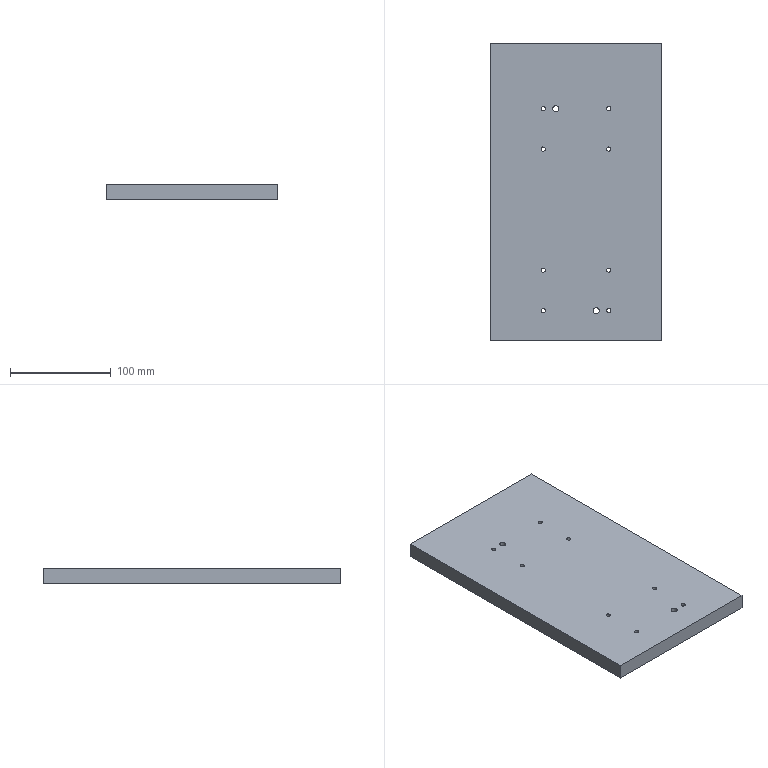Part | STEP file | SN10_012_002_PLACA | 1 solid | 16 faces | box 170 x 295 x 15 mm | volume 749791 mm3 | cylinder 10 | plane 6 | commonest cylinder face diameters 4.134 x8 6 x2
STEP:
#1=CARTESIAN_POINT('',(0.,0.,0.));
#2=DIRECTION('',(0.,0.,1.));
#3=DIRECTION('',(1.,0.,0.));
#4=AXIS2_PLACEMENT_3D('',#1,#2,#3);
#5=CARTESIAN_POINT('',(156.943,249.009,60.));
#6=VERTEX_POINT('',#5);
#7=CARTESIAN_POINT('',(155.129,250.,60.));
#8=DIRECTION('',(0.,0.,1.));
#9=DIRECTION('',(1.,0.,0.));
#10=AXIS2_PLACEMENT_3D('',#7,#8,#9);
#11=CIRCLE('',#10,2.067);
#12=CARTESIAN_POINT('',(155.129,250.,59.9));
#13=DIRECTION('',(0.,0.,-1.));
#14=DIRECTION('',(0.8776,-0.4794,0.));
#15=AXIS2_PLACEMENT_3D('',#12,#13,#14);
#16=CYLINDRICAL_SURFACE('',#15,2.067);
#17=CARTESIAN_POINT('',(12.066,-0.1));
#18=DIRECTION('',(-1.,0.));
#19=VECTOR('',#18,1.);
#20=LINE('',#17,#19);
#21=(GEOMETRIC_REPRESENTATION_CONTEXT(2)PARAMETRIC_REPRESENTATION_CONTEXT()REPRESENTATION_CONTEXT('',''));
#22=DEFINITIONAL_REPRESENTATION('',(#20),#21);
#23=PCURVE('',#16,#22);
#24=CARTESIAN_POINT('',(0.,0.,60.));
#25=DIRECTION('',(0.,0.,1.));
#26=DIRECTION('',(1.,0.,0.));
#27=AXIS2_PLACEMENT_3D('',#24,#25,#26);
#28=PLANE('',#27);
#29=CARTESIAN_POINT('',(155.129,250.));
#30=DIRECTION('',(1.,0.));
#31=AXIS2_PLACEMENT_2D('',#29,#30);
#32=CIRCLE('',#31,2.067);
#33=(GEOMETRIC_REPRESENTATION_CONTEXT(2)PARAMETRIC_REPRESENTATION_CONTEXT()REPRESENTATION_CONTEXT('',''));
#34=DEFINITIONAL_REPRESENTATION('',(#32),#33);
#35=PCURVE('',#28,#34);
#36=SURFACE_CURVE('',#11,(#23,#35),.PCURVE_S1.);
#37=EDGE_CURVE('',#6,#6,#36,.T.);
#38=ORIENTED_EDGE('',*,*,#37,.F.);
#39=CARTESIAN_POINT('',(156.943,249.009,45.));
#40=VERTEX_POINT('',#39);
#41=CARTESIAN_POINT('',(156.943,249.009,60.));
#42=CARTESIAN_POINT('',(156.943,249.009,45.));
#43=B_SPLINE_CURVE_WITH_KNOTS('',1,(#41,#42),.UNSPECIFIED.,.F.,.F.,(2,2),(-0.1,14.9),.PIECEWISE_BEZIER_KNOTS.);
#44=CARTESIAN_POINT('',(6.283,0.));
#45=DIRECTION('',(0.,1.));
#46=VECTOR('',#45,1.);
#47=LINE('',#44,#46);
#48=(GEOMETRIC_REPRESENTATION_CONTEXT(2)PARAMETRIC_REPRESENTATION_CONTEXT()REPRESENTATION_CONTEXT('',''));
#49=DEFINITIONAL_REPRESENTATION('',(#47),#48);
#50=PCURVE('',#16,#49);
#51=CARTESIAN_POINT('',(0.,0.));
#52=DIRECTION('',(0.,1.));
#53=VECTOR('',#52,1.);
#54=LINE('',#51,#53);
#55=(GEOMETRIC_REPRESENTATION_CONTEXT(2)PARAMETRIC_REPRESENTATION_CONTEXT()REPRESENTATION_CONTEXT('',''));
#56=DEFINITIONAL_REPRESENTATION('',(#54),#55);
#57=PCURVE('',#16,#56);
#58=SEAM_CURVE('',#43,(#50,#57),.PCURVE_S1.);
#59=EDGE_CURVE('',#6,#40,#58,.T.);
#60=ORIENTED_EDGE('',*,*,#59,.T.);
#61=CARTESIAN_POINT('',(155.129,250.,45.));
#62=DIRECTION('',(0.,0.,-1.));
#63=DIRECTION('',(1.,0.,0.));
#64=AXIS2_PLACEMENT_3D('',#61,#62,#63);
#65=CIRCLE('',#64,2.067);
#66=CARTESIAN_POINT('',(-0.5,14.9));
#67=DIRECTION('',(1.,0.));
#68=VECTOR('',#67,1.);
#69=LINE('',#66,#68);
#70=(GEOMETRIC_REPRESENTATION_CONTEXT(2)PARAMETRIC_REPRESENTATION_CONTEXT()REPRESENTATION_CONTEXT('',''));
#71=DEFINITIONAL_REPRESENTATION('',(#69),#70);
#72=PCURVE('',#16,#71);
#73=CARTESIAN_POINT('',(0.,0.,45.));
#74=DIRECTION('',(0.,0.,1.));
#75=DIRECTION('',(1.,0.,0.));
#76=AXIS2_PLACEMENT_3D('',#73,#74,#75);
#77=PLANE('',#76);
#78=CARTESIAN_POINT('',(157.196,250.));
#79=CARTESIAN_POINT('',(157.196,246.42));
#80=CARTESIAN_POINT('',(154.095,248.21));
#81=CARTESIAN_POINT('',(150.995,250.));
#82=CARTESIAN_POINT('',(154.095,251.79));
#83=CARTESIAN_POINT('',(157.196,253.58));
#84=CARTESIAN_POINT('',(157.196,250.));
#85=(BOUNDED_CURVE()B_SPLINE_CURVE(2,(#78,#79,#80,#81,#82,#83,#84),.UNSPECIFIED.,.T.,.F.)B_SPLINE_CURVE_WITH_KNOTS((1,2,2,2,2,1),(-2.094,0.,2.094,4.189,6.283,8.378),.UNSPECIFIED.)CURVE()GEOMETRIC_REPRESENTATION_ITEM()RATIONAL_B_SPLINE_CURVE((1.,0.5,1.,0.5,1.,0.5,1.))REPRESENTATION_ITEM(''));
#86=(GEOMETRIC_REPRESENTATION_CONTEXT(2)PARAMETRIC_REPRESENTATION_CONTEXT()REPRESENTATION_CONTEXT('',''));
#87=DEFINITIONAL_REPRESENTATION('',(#85),#86);
#88=PCURVE('',#77,#87);
#89=SURFACE_CURVE('',#65,(#72,#88),.PCURVE_S1.);
#90=EDGE_CURVE('',#40,#40,#89,.T.);
#91=ORIENTED_EDGE('',*,*,#90,.F.);
#92=ORIENTED_EDGE('',*,*,#59,.F.);
#93=EDGE_LOOP('',(#38,#60,#91,#92));
#94=FACE_BOUND('',#93,.F.);
#95=ADVANCED_FACE('',(#94),#16,.F.);
#96=CARTESIAN_POINT('',(102.629,475.,60.));
#97=VERTEX_POINT('',#96);
#98=CARTESIAN_POINT('',(102.629,180.,60.));
#99=VERTEX_POINT('',#98);
#100=CARTESIAN_POINT('',(102.629,475.,60.));
#101=DIRECTION('',(0.,-1.,0.));
#102=VECTOR('',#101,1.);
#103=LINE('',#100,#102);
#104=CARTESIAN_POINT('',(102.629,475.));
#105=DIRECTION('',(0.,-1.));
#106=VECTOR('',#105,1.);
#107=LINE('',#104,#106);
#108=(GEOMETRIC_REPRESENTATION_CONTEXT(2)PARAMETRIC_REPRESENTATION_CONTEXT()REPRESENTATION_CONTEXT('',''));
#109=DEFINITIONAL_REPRESENTATION('',(#107),#108);
#110=PCURVE('',#28,#109);
#111=CARTESIAN_POINT('',(102.629,475.,45.));
#112=DIRECTION('',(-1.,0.,0.));
#113=DIRECTION('',(0.,0.,1.));
#114=AXIS2_PLACEMENT_3D('',#111,#112,#113);
#115=PLANE('',#114);
#116=CARTESIAN_POINT('',(15.,0.));
#117=DIRECTION('',(0.,-1.));
#118=VECTOR('',#117,1.);
#119=LINE('',#116,#118);
#120=(GEOMETRIC_REPRESENTATION_CONTEXT(2)PARAMETRIC_REPRESENTATION_CONTEXT()REPRESENTATION_CONTEXT('',''));
#121=DEFINITIONAL_REPRESENTATION('',(#119),#120);
#122=PCURVE('',#115,#121);
#123=SURFACE_CURVE('',#103,(#110,#122),.PCURVE_S1.);
#124=EDGE_CURVE('',#97,#99,#123,.T.);
#125=ORIENTED_EDGE('',*,*,#124,.T.);
#126=CARTESIAN_POINT('',(272.629,180.,60.));
#127=VERTEX_POINT('',#126);
#128=CARTESIAN_POINT('',(272.629,180.,60.));
#129=DIRECTION('',(-1.,0.,0.));
#130=VECTOR('',#129,1.);
#131=LINE('',#128,#130);
#132=CARTESIAN_POINT('',(272.629,180.));
#133=DIRECTION('',(-1.,0.));
#134=VECTOR('',#133,1.);
#135=LINE('',#132,#134);
#136=(GEOMETRIC_REPRESENTATION_CONTEXT(2)PARAMETRIC_REPRESENTATION_CONTEXT()REPRESENTATION_CONTEXT('',''));
#137=DEFINITIONAL_REPRESENTATION('',(#135),#136);
#138=PCURVE('',#28,#137);
#139=CARTESIAN_POINT('',(272.629,180.,45.));
#140=DIRECTION('',(0.,1.,0.));
#141=DIRECTION('',(0.,0.,1.));
#142=AXIS2_PLACEMENT_3D('',#139,#140,#141);
#143=PLANE('',#142);
#144=CARTESIAN_POINT('',(15.,0.));
#145=DIRECTION('',(0.,-1.));
#146=VECTOR('',#145,1.);
#147=LINE('',#144,#146);
#148=(GEOMETRIC_REPRESENTATION_CONTEXT(2)PARAMETRIC_REPRESENTATION_CONTEXT()REPRESENTATION_CONTEXT('',''));
#149=DEFINITIONAL_REPRESENTATION('',(#147),#148);
#150=PCURVE('',#143,#149);
#151=SURFACE_CURVE('',#131,(#138,#150),.PCURVE_S1.);
#152=EDGE_CURVE('',#127,#99,#151,.T.);
#153=ORIENTED_EDGE('',*,*,#152,.F.);
#154=CARTESIAN_POINT('',(272.629,475.,60.));
#155=VERTEX_POINT('',#154);
#156=CARTESIAN_POINT('',(272.629,180.,60.));
#157=DIRECTION('',(0.,1.,0.));
#158=VECTOR('',#157,1.);
#159=LINE('',#156,#158);
#160=CARTESIAN_POINT('',(272.629,180.));
#161=DIRECTION('',(0.,1.));
#162=VECTOR('',#161,1.);
#163=LINE('',#160,#162);
#164=(GEOMETRIC_REPRESENTATION_CONTEXT(2)PARAMETRIC_REPRESENTATION_CONTEXT()REPRESENTATION_CONTEXT('',''));
#165=DEFINITIONAL_REPRESENTATION('',(#163),#164);
#166=PCURVE('',#28,#165);
#167=CARTESIAN_POINT('',(272.629,180.,45.));
#168=DIRECTION('',(1.,0.,0.));
#169=DIRECTION('',(0.,0.,-1.));
#170=AXIS2_PLACEMENT_3D('',#167,#168,#169);
#171=PLANE('',#170);
#172=CARTESIAN_POINT('',(-15.,0.));
#173=DIRECTION('',(0.,1.));
#174=VECTOR('',#173,1.);
#175=LINE('',#172,#174);
#176=(GEOMETRIC_REPRESENTATION_CONTEXT(2)PARAMETRIC_REPRESENTATION_CONTEXT()REPRESENTATION_CONTEXT('',''));
#177=DEFINITIONAL_REPRESENTATION('',(#175),#176);
#178=PCURVE('',#171,#177);
#179=SURFACE_CURVE('',#159,(#166,#178),.PCURVE_S1.);
#180=EDGE_CURVE('',#127,#155,#179,.T.);
#181=ORIENTED_EDGE('',*,*,#180,.T.);
#182=CARTESIAN_POINT('',(102.629,475.,60.));
#183=DIRECTION('',(1.,0.,0.));
#184=VECTOR('',#183,1.);
#185=LINE('',#182,#184);
#186=CARTESIAN_POINT('',(102.629,475.));
#187=DIRECTION('',(1.,0.));
#188=VECTOR('',#187,1.);
#189=LINE('',#186,#188);
#190=(GEOMETRIC_REPRESENTATION_CONTEXT(2)PARAMETRIC_REPRESENTATION_CONTEXT()REPRESENTATION_CONTEXT('',''));
#191=DEFINITIONAL_REPRESENTATION('',(#189),#190);
#192=PCURVE('',#28,#191);
#193=CARTESIAN_POINT('',(102.629,475.,45.));
#194=DIRECTION('',(0.,-1.,0.));
#195=DIRECTION('',(0.,0.,-1.));
#196=AXIS2_PLACEMENT_3D('',#193,#194,#195);
#197=PLANE('',#196);
#198=CARTESIAN_POINT('',(-15.,0.));
#199=DIRECTION('',(0.,1.));
#200=VECTOR('',#199,1.);
#201=LINE('',#198,#200);
#202=(GEOMETRIC_REPRESENTATION_CONTEXT(2)PARAMETRIC_REPRESENTATION_CONTEXT()REPRESENTATION_CONTEXT('',''));
#203=DEFINITIONAL_REPRESENTATION('',(#201),#202);
#204=PCURVE('',#197,#203);
#205=SURFACE_CURVE('',#185,(#192,#204),.PCURVE_S1.);
#206=EDGE_CURVE('',#97,#155,#205,.T.);
#207=ORIENTED_EDGE('',*,*,#206,.F.);
#208=EDGE_LOOP('',(#125,#153,#181,#207));
#209=FACE_BOUND('',#208,.T.);
#210=ORIENTED_EDGE('',*,*,#37,.F.);
#211=EDGE_LOOP('',(#210));
#212=FACE_BOUND('',#211,.T.);
#213=CARTESIAN_POINT('',(156.943,209.009,60.));
#214=VERTEX_POINT('',#213);
#215=CARTESIAN_POINT('',(155.129,210.,60.));
#216=DIRECTION('',(0.,0.,1.));
#217=DIRECTION('',(1.,0.,0.));
#218=AXIS2_PLACEMENT_3D('',#215,#216,#217);
#219=CIRCLE('',#218,2.067);
#220=CARTESIAN_POINT('',(155.129,210.));
#221=DIRECTION('',(1.,0.));
#222=AXIS2_PLACEMENT_2D('',#220,#221);
#223=CIRCLE('',#222,2.067);
#224=(GEOMETRIC_REPRESENTATION_CONTEXT(2)PARAMETRIC_REPRESENTATION_CONTEXT()REPRESENTATION_CONTEXT('',''));
#225=DEFINITIONAL_REPRESENTATION('',(#223),#224);
#226=PCURVE('',#28,#225);
#227=CARTESIAN_POINT('',(155.129,210.,59.9));
#228=DIRECTION('',(0.,0.,-1.));
#229=DIRECTION('',(0.8776,-0.4794,0.));
#230=AXIS2_PLACEMENT_3D('',#227,#228,#229);
#231=CYLINDRICAL_SURFACE('',#230,2.067);
#232=CARTESIAN_POINT('',(12.066,-0.1));
#233=DIRECTION('',(-1.,0.));
#234=VECTOR('',#233,1.);
#235=LINE('',#232,#234);
#236=(GEOMETRIC_REPRESENTATION_CONTEXT(2)PARAMETRIC_REPRESENTATION_CONTEXT()REPRESENTATION_CONTEXT('',''));
#237=DEFINITIONAL_REPRESENTATION('',(#235),#236);
#238=PCURVE('',#231,#237);
#239=SURFACE_CURVE('',#219,(#226,#238),.PCURVE_S1.);
#240=EDGE_CURVE('',#214,#214,#239,.T.);
#241=ORIENTED_EDGE('',*,*,#240,.F.);
#242=EDGE_LOOP('',(#241));
#243=FACE_BOUND('',#242,.T.);
#244=CARTESIAN_POINT('',(221.943,209.009,60.));
#245=VERTEX_POINT('',#244);
#246=CARTESIAN_POINT('',(220.129,210.,60.));
#247=DIRECTION('',(0.,0.,1.));
#248=DIRECTION('',(1.,0.,0.));
#249=AXIS2_PLACEMENT_3D('',#246,#247,#248);
#250=CIRCLE('',#249,2.067);
#251=CARTESIAN_POINT('',(220.129,210.));
#252=DIRECTION('',(1.,0.));
#253=AXIS2_PLACEMENT_2D('',#251,#252);
#254=CIRCLE('',#253,2.067);
#255=(GEOMETRIC_REPRESENTATION_CONTEXT(2)PARAMETRIC_REPRESENTATION_CONTEXT()REPRESENTATION_CONTEXT('',''));
#256=DEFINITIONAL_REPRESENTATION('',(#254),#255);
#257=PCURVE('',#28,#256);
#258=CARTESIAN_POINT('',(220.129,210.,59.9));
#259=DIRECTION('',(0.,0.,-1.));
#260=DIRECTION('',(0.8776,-0.4794,0.));
#261=AXIS2_PLACEMENT_3D('',#258,#259,#260);
#262=CYLINDRICAL_SURFACE('',#261,2.067);
#263=CARTESIAN_POINT('',(12.066,-0.1));
#264=DIRECTION('',(-1.,0.));
#265=VECTOR('',#264,1.);
#266=LINE('',#263,#265);
#267=(GEOMETRIC_REPRESENTATION_CONTEXT(2)PARAMETRIC_REPRESENTATION_CONTEXT()REPRESENTATION_CONTEXT('',''));
#268=DEFINITIONAL_REPRESENTATION('',(#266),#267);
#269=PCURVE('',#262,#268);
#270=SURFACE_CURVE('',#250,(#257,#269),.PCURVE_S1.);
#271=EDGE_CURVE('',#245,#245,#270,.T.);
#272=ORIENTED_EDGE('',*,*,#271,.F.);
#273=EDGE_LOOP('',(#272));
#274=FACE_BOUND('',#273,.T.);
#275=CARTESIAN_POINT('',(221.943,249.009,60.));
#276=VERTEX_POINT('',#275);
#277=CARTESIAN_POINT('',(220.129,250.,60.));
#278=DIRECTION('',(0.,0.,1.));
#279=DIRECTION('',(1.,0.,0.));
#280=AXIS2_PLACEMENT_3D('',#277,#278,#279);
#281=CIRCLE('',#280,2.067);
#282=CARTESIAN_POINT('',(220.129,250.));
#283=DIRECTION('',(1.,0.));
#284=AXIS2_PLACEMENT_2D('',#282,#283);
#285=CIRCLE('',#284,2.067);
#286=(GEOMETRIC_REPRESENTATION_CONTEXT(2)PARAMETRIC_REPRESENTATION_CONTEXT()REPRESENTATION_CONTEXT('',''));
#287=DEFINITIONAL_REPRESENTATION('',(#285),#286);
#288=PCURVE('',#28,#287);
#289=CARTESIAN_POINT('',(220.129,250.,59.9));
#290=DIRECTION('',(0.,0.,-1.));
#291=DIRECTION('',(0.8776,-0.4794,0.));
#292=AXIS2_PLACEMENT_3D('',#289,#290,#291);
#293=CYLINDRICAL_SURFACE('',#292,2.067);
#294=CARTESIAN_POINT('',(12.066,-0.1));
#295=DIRECTION('',(-1.,0.));
#296=VECTOR('',#295,1.);
#297=LINE('',#294,#296);
#298=(GEOMETRIC_REPRESENTATION_CONTEXT(2)PARAMETRIC_REPRESENTATION_CONTEXT()REPRESENTATION_CONTEXT('',''));
#299=DEFINITIONAL_REPRESENTATION('',(#297),#298);
#300=PCURVE('',#293,#299);
#301=SURFACE_CURVE('',#281,(#288,#300),.PCURVE_S1.);
#302=EDGE_CURVE('',#276,#276,#301,.T.);
#303=ORIENTED_EDGE('',*,*,#302,.F.);
#304=EDGE_LOOP('',(#303));
#305=FACE_BOUND('',#304,.T.);
#306=CARTESIAN_POINT('',(221.943,369.009,60.));
#307=VERTEX_POINT('',#306);
#308=CARTESIAN_POINT('',(220.129,370.,60.));
#309=DIRECTION('',(0.,0.,1.));
#310=DIRECTION('',(1.,0.,0.));
#311=AXIS2_PLACEMENT_3D('',#308,#309,#310);
#312=CIRCLE('',#311,2.067);
#313=CARTESIAN_POINT('',(220.129,370.));
#314=DIRECTION('',(1.,0.));
#315=AXIS2_PLACEMENT_2D('',#313,#314);
#316=CIRCLE('',#315,2.067);
#317=(GEOMETRIC_REPRESENTATION_CONTEXT(2)PARAMETRIC_REPRESENTATION_CONTEXT()REPRESENTATION_CONTEXT('',''));
#318=DEFINITIONAL_REPRESENTATION('',(#316),#317);
#319=PCURVE('',#28,#318);
#320=CARTESIAN_POINT('',(220.129,370.,59.9));
#321=DIRECTION('',(0.,0.,-1.));
#322=DIRECTION('',(0.8776,-0.4794,0.));
#323=AXIS2_PLACEMENT_3D('',#320,#321,#322);
#324=CYLINDRICAL_SURFACE('',#323,2.067);
#325=CARTESIAN_POINT('',(12.066,-0.1));
#326=DIRECTION('',(-1.,0.));
#327=VECTOR('',#326,1.);
#328=LINE('',#325,#327);
#329=(GEOMETRIC_REPRESENTATION_CONTEXT(2)PARAMETRIC_REPRESENTATION_CONTEXT()REPRESENTATION_CONTEXT('',''));
#330=DEFINITIONAL_REPRESENTATION('',(#328),#329);
#331=PCURVE('',#324,#330);
#332=SURFACE_CURVE('',#312,(#319,#331),.PCURVE_S1.);
#333=EDGE_CURVE('',#307,#307,#332,.T.);
#334=ORIENTED_EDGE('',*,*,#333,.F.);
#335=EDGE_LOOP('',(#334));
#336=FACE_BOUND('',#335,.T.);
#337=CARTESIAN_POINT('',(156.943,369.009,60.));
#338=VERTEX_POINT('',#337);
#339=CARTESIAN_POINT('',(155.129,370.,60.));
#340=DIRECTION('',(0.,0.,1.));
#341=DIRECTION('',(1.,0.,0.));
#342=AXIS2_PLACEMENT_3D('',#339,#340,#341);
#343=CIRCLE('',#342,2.067);
#344=CARTESIAN_POINT('',(155.129,370.));
#345=DIRECTION('',(1.,0.));
#346=AXIS2_PLACEMENT_2D('',#344,#345);
#347=CIRCLE('',#346,2.067);
#348=(GEOMETRIC_REPRESENTATION_CONTEXT(2)PARAMETRIC_REPRESENTATION_CONTEXT()REPRESENTATION_CONTEXT('',''));
#349=DEFINITIONAL_REPRESENTATION('',(#347),#348);
#350=PCURVE('',#28,#349);
#351=CARTESIAN_POINT('',(155.129,370.,59.9));
#352=DIRECTION('',(0.,0.,-1.));
#353=DIRECTION('',(0.8776,-0.4794,0.));
#354=AXIS2_PLACEMENT_3D('',#351,#352,#353);
#355=CYLINDRICAL_SURFACE('',#354,2.067);
#356=CARTESIAN_POINT('',(12.066,-0.1));
#357=DIRECTION('',(-1.,0.));
#358=VECTOR('',#357,1.);
#359=LINE('',#356,#358);
#360=(GEOMETRIC_REPRESENTATION_CONTEXT(2)PARAMETRIC_REPRESENTATION_CONTEXT()REPRESENTATION_CONTEXT('',''));
#361=DEFINITIONAL_REPRESENTATION('',(#359),#360);
#362=PCURVE('',#355,#361);
#363=SURFACE_CURVE('',#343,(#350,#362),.PCURVE_S1.);
#364=EDGE_CURVE('',#338,#338,#363,.T.);
#365=ORIENTED_EDGE('',*,*,#364,.F.);
#366=EDGE_LOOP('',(#365));
#367=FACE_BOUND('',#366,.T.);
#368=CARTESIAN_POINT('',(156.943,409.009,60.));
#369=VERTEX_POINT('',#368);
#370=CARTESIAN_POINT('',(155.129,410.,60.));
#371=DIRECTION('',(0.,0.,1.));
#372=DIRECTION('',(1.,0.,0.));
#373=AXIS2_PLACEMENT_3D('',#370,#371,#372);
#374=CIRCLE('',#373,2.067);
#375=CARTESIAN_POINT('',(155.129,410.));
#376=DIRECTION('',(1.,0.));
#377=AXIS2_PLACEMENT_2D('',#375,#376);
#378=CIRCLE('',#377,2.067);
#379=(GEOMETRIC_REPRESENTATION_CONTEXT(2)PARAMETRIC_REPRESENTATION_CONTEXT()REPRESENTATION_CONTEXT('',''));
#380=DEFINITIONAL_REPRESENTATION('',(#378),#379);
#381=PCURVE('',#28,#380);
#382=CARTESIAN_POINT('',(155.129,410.,59.9));
#383=DIRECTION('',(0.,0.,-1.));
#384=DIRECTION('',(0.8776,-0.4794,0.));
#385=AXIS2_PLACEMENT_3D('',#382,#383,#384);
#386=CYLINDRICAL_SURFACE('',#385,2.067);
#387=CARTESIAN_POINT('',(12.066,-0.1));
#388=DIRECTION('',(-1.,0.));
#389=VECTOR('',#388,1.);
#390=LINE('',#387,#389);
#391=(GEOMETRIC_REPRESENTATION_CONTEXT(2)PARAMETRIC_REPRESENTATION_CONTEXT()REPRESENTATION_CONTEXT('',''));
#392=DEFINITIONAL_REPRESENTATION('',(#390),#391);
#393=PCURVE('',#386,#392);
#394=SURFACE_CURVE('',#374,(#381,#393),.PCURVE_S1.);
#395=EDGE_CURVE('',#369,#369,#394,.T.);
#396=ORIENTED_EDGE('',*,*,#395,.F.);
#397=EDGE_LOOP('',(#396));
#398=FACE_BOUND('',#397,.T.);
#399=CARTESIAN_POINT('',(221.943,409.009,60.));
#400=VERTEX_POINT('',#399);
#401=CARTESIAN_POINT('',(220.129,410.,60.));
#402=DIRECTION('',(0.,0.,1.));
#403=DIRECTION('',(1.,0.,0.));
#404=AXIS2_PLACEMENT_3D('',#401,#402,#403);
#405=CIRCLE('',#404,2.067);
#406=CARTESIAN_POINT('',(220.129,410.));
#407=DIRECTION('',(1.,0.));
#408=AXIS2_PLACEMENT_2D('',#406,#407);
#409=CIRCLE('',#408,2.067);
#410=(GEOMETRIC_REPRESENTATION_CONTEXT(2)PARAMETRIC_REPRESENTATION_CONTEXT()REPRESENTATION_CONTEXT('',''));
#411=DEFINITIONAL_REPRESENTATION('',(#409),#410);
#412=PCURVE('',#28,#411);
#413=CARTESIAN_POINT('',(220.129,410.,59.9));
#414=DIRECTION('',(0.,0.,-1.));
#415=DIRECTION('',(0.8776,-0.4794,0.));
#416=AXIS2_PLACEMENT_3D('',#413,#414,#415);
#417=CYLINDRICAL_SURFACE('',#416,2.067);
#418=CARTESIAN_POINT('',(12.066,-0.1));
#419=DIRECTION('',(-1.,0.));
#420=VECTOR('',#419,1.);
#421=LINE('',#418,#420);
#422=(GEOMETRIC_REPRESENTATION_CONTEXT(2)PARAMETRIC_REPRESENTATION_CONTEXT()REPRESENTATION_CONTEXT('',''));
#423=DEFINITIONAL_REPRESENTATION('',(#421),#422);
#424=PCURVE('',#417,#423);
#425=SURFACE_CURVE('',#405,(#412,#424),.PCURVE_S1.);
#426=EDGE_CURVE('',#400,#400,#425,.T.);
#427=ORIENTED_EDGE('',*,*,#426,.F.);
#428=EDGE_LOOP('',(#427));
#429=FACE_BOUND('',#428,.T.);
#430=CARTESIAN_POINT('',(210.262,208.562,60.));
#431=VERTEX_POINT('',#430);
#432=CARTESIAN_POINT('',(207.629,210.,60.));
#433=DIRECTION('',(0.,0.,1.));
#434=DIRECTION('',(1.,0.,0.));
#435=AXIS2_PLACEMENT_3D('',#432,#433,#434);
#436=CIRCLE('',#435,3.);
#437=CARTESIAN_POINT('',(207.629,210.));
#438=DIRECTION('',(1.,0.));
#439=AXIS2_PLACEMENT_2D('',#437,#438);
#440=CIRCLE('',#439,3.);
#441=(GEOMETRIC_REPRESENTATION_CONTEXT(2)PARAMETRIC_REPRESENTATION_CONTEXT()REPRESENTATION_CONTEXT('',''));
#442=DEFINITIONAL_REPRESENTATION('',(#440),#441);
#443=PCURVE('',#28,#442);
#444=CARTESIAN_POINT('',(207.629,210.,59.9));
#445=DIRECTION('',(0.,0.,-1.));
#446=DIRECTION('',(0.8776,-0.4794,0.));
#447=AXIS2_PLACEMENT_3D('',#444,#445,#446);
#448=CYLINDRICAL_SURFACE('',#447,3.);
#449=CARTESIAN_POINT('',(12.066,-0.1));
#450=DIRECTION('',(-1.,0.));
#451=VECTOR('',#450,1.);
#452=LINE('',#449,#451);
#453=(GEOMETRIC_REPRESENTATION_CONTEXT(2)PARAMETRIC_REPRESENTATION_CONTEXT()REPRESENTATION_CONTEXT('',''));
#454=DEFINITIONAL_REPRESENTATION('',(#452),#453);
#455=PCURVE('',#448,#454);
#456=SURFACE_CURVE('',#436,(#443,#455),.PCURVE_S1.);
#457=EDGE_CURVE('',#431,#431,#456,.T.);
#458=ORIENTED_EDGE('',*,*,#457,.F.);
#459=EDGE_LOOP('',(#458));
#460=FACE_BOUND('',#459,.T.);
#461=CARTESIAN_POINT('',(170.262,408.562,60.));
#462=VERTEX_POINT('',#461);
#463=CARTESIAN_POINT('',(167.629,410.,60.));
#464=DIRECTION('',(0.,0.,1.));
#465=DIRECTION('',(1.,0.,0.));
#466=AXIS2_PLACEMENT_3D('',#463,#464,#465);
#467=CIRCLE('',#466,3.);
#468=CARTESIAN_POINT('',(167.629,410.));
#469=DIRECTION('',(1.,0.));
#470=AXIS2_PLACEMENT_2D('',#468,#469);
#471=CIRCLE('',#470,3.);
#472=(GEOMETRIC_REPRESENTATION_CONTEXT(2)PARAMETRIC_REPRESENTATION_CONTEXT()REPRESENTATION_CONTEXT('',''));
#473=DEFINITIONAL_REPRESENTATION('',(#471),#472);
#474=PCURVE('',#28,#473);
#475=CARTESIAN_POINT('',(167.629,410.,59.9));
#476=DIRECTION('',(0.,0.,-1.));
#477=DIRECTION('',(0.8776,-0.4794,0.));
#478=AXIS2_PLACEMENT_3D('',#475,#476,#477);
#479=CYLINDRICAL_SURFACE('',#478,3.);
#480=CARTESIAN_POINT('',(12.066,-0.1));
#481=DIRECTION('',(-1.,0.));
#482=VECTOR('',#481,1.);
#483=LINE('',#480,#482);
#484=(GEOMETRIC_REPRESENTATION_CONTEXT(2)PARAMETRIC_REPRESENTATION_CONTEXT()REPRESENTATION_CONTEXT('',''));
#485=DEFINITIONAL_REPRESENTATION('',(#483),#484);
#486=PCURVE('',#479,#485);
#487=SURFACE_CURVE('',#467,(#474,#486),.PCURVE_S1.);
#488=EDGE_CURVE('',#462,#462,#487,.T.);
#489=ORIENTED_EDGE('',*,*,#488,.F.);
#490=EDGE_LOOP('',(#489));
#491=FACE_BOUND('',#490,.T.);
#492=ADVANCED_FACE('',(#209,#212,#243,#274,#305,#336,#367,#398,#429,#460,#491),#28,.T.);
#493=CARTESIAN_POINT('',(102.629,475.,45.));
#494=VERTEX_POINT('',#493);
#495=CARTESIAN_POINT('',(102.629,475.,45.));
#496=DIRECTION('',(0.,0.,1.));
#497=VECTOR('',#496,1.);
#498=LINE('',#495,#497);
#499=CARTESIAN_POINT('',(0.,0.));
#500=DIRECTION('',(1.,0.));
#501=VECTOR('',#500,1.);
#502=LINE('',#499,#501);
#503=(GEOMETRIC_REPRESENTATION_CONTEXT(2)PARAMETRIC_REPRESENTATION_CONTEXT()REPRESENTATION_CONTEXT('',''));
#504=DEFINITIONAL_REPRESENTATION('',(#502),#503);
#505=PCURVE('',#115,#504);
#506=CARTESIAN_POINT('',(0.,0.));
#507=DIRECTION('',(-1.,0.));
#508=VECTOR('',#507,1.);
#509=LINE('',#506,#508);
#510=(GEOMETRIC_REPRESENTATION_CONTEXT(2)PARAMETRIC_REPRESENTATION_CONTEXT()REPRESENTATION_CONTEXT('',''));
#511=DEFINITIONAL_REPRESENTATION('',(#509),#510);
#512=PCURVE('',#197,#511);
#513=SURFACE_CURVE('',#498,(#505,#512),.PCURVE_S1.);
#514=EDGE_CURVE('',#494,#97,#513,.T.);
#515=ORIENTED_EDGE('',*,*,#514,.F.);
#516=CARTESIAN_POINT('',(102.629,180.,45.));
#517=VERTEX_POINT('',#516);
#518=CARTESIAN_POINT('',(102.629,475.,45.));
#519=DIRECTION('',(0.,-1.,0.));
#520=VECTOR('',#519,1.);
#521=LINE('',#518,#520);
#522=CARTESIAN_POINT('',(0.,0.));
#523=DIRECTION('',(0.,-1.));
#524=VECTOR('',#523,1.);
#525=LINE('',#522,#524);
#526=(GEOMETRIC_REPRESENTATION_CONTEXT(2)PARAMETRIC_REPRESENTATION_CONTEXT()REPRESENTATION_CONTEXT('',''));
#527=DEFINITIONAL_REPRESENTATION('',(#525),#526);
#528=PCURVE('',#115,#527);
#529=CARTESIAN_POINT('',(102.629,475.));
#530=DIRECTION('',(0.,-1.));
#531=VECTOR('',#530,1.);
#532=LINE('',#529,#531);
#533=(GEOMETRIC_REPRESENTATION_CONTEXT(2)PARAMETRIC_REPRESENTATION_CONTEXT()REPRESENTATION_CONTEXT('',''));
#534=DEFINITIONAL_REPRESENTATION('',(#532),#533);
#535=PCURVE('',#77,#534);
#536=SURFACE_CURVE('',#521,(#528,#535),.PCURVE_S1.);
#537=EDGE_CURVE('',#494,#517,#536,.T.);
#538=ORIENTED_EDGE('',*,*,#537,.T.);
#539=CARTESIAN_POINT('',(102.629,180.,45.));
#540=DIRECTION('',(0.,0.,1.));
#541=VECTOR('',#540,1.);
#542=LINE('',#539,#541);
#543=CARTESIAN_POINT('',(0.,-295.));
#544=DIRECTION('',(1.,0.));
#545=VECTOR('',#544,1.);
#546=LINE('',#543,#545);
#547=(GEOMETRIC_REPRESENTATION_CONTEXT(2)PARAMETRIC_REPRESENTATION_CONTEXT()REPRESENTATION_CONTEXT('',''));
#548=DEFINITIONAL_REPRESENTATION('',(#546),#547);
#549=PCURVE('',#115,#548);
#550=CARTESIAN_POINT('',(0.,-170.));
#551=DIRECTION('',(1.,0.));
#552=VECTOR('',#551,1.);
#553=LINE('',#550,#552);
#554=(GEOMETRIC_REPRESENTATION_CONTEXT(2)PARAMETRIC_REPRESENTATION_CONTEXT()REPRESENTATION_CONTEXT('',''));
#555=DEFINITIONAL_REPRESENTATION('',(#553),#554);
#556=PCURVE('',#143,#555);
#557=SURFACE_CURVE('',#542,(#549,#556),.PCURVE_S1.);
#558=EDGE_CURVE('',#517,#99,#557,.T.);
#559=ORIENTED_EDGE('',*,*,#558,.T.);
#560=ORIENTED_EDGE('',*,*,#124,.F.);
#561=EDGE_LOOP('',(#515,#538,#559,#560));
#562=FACE_BOUND('',#561,.T.);
#563=ADVANCED_FACE('',(#562),#115,.T.);
#564=ORIENTED_EDGE('',*,*,#558,.F.);
#565=CARTESIAN_POINT('',(272.629,180.,45.));
#566=VERTEX_POINT('',#565);
#567=CARTESIAN_POINT('',(272.629,180.,45.));
#568=DIRECTION('',(-1.,0.,0.));
#569=VECTOR('',#568,1.);
#570=LINE('',#567,#569);
#571=CARTESIAN_POINT('',(0.,0.));
#572=DIRECTION('',(0.,-1.));
#573=VECTOR('',#572,1.);
#574=LINE('',#571,#573);
#575=(GEOMETRIC_REPRESENTATION_CONTEXT(2)PARAMETRIC_REPRESENTATION_CONTEXT()REPRESENTATION_CONTEXT('',''));
#576=DEFINITIONAL_REPRESENTATION('',(#574),#575);
#577=PCURVE('',#143,#576);
#578=CARTESIAN_POINT('',(272.629,180.));
#579=DIRECTION('',(-1.,0.));
#580=VECTOR('',#579,1.);
#581=LINE('',#578,#580);
#582=(GEOMETRIC_REPRESENTATION_CONTEXT(2)PARAMETRIC_REPRESENTATION_CONTEXT()REPRESENTATION_CONTEXT('',''));
#583=DEFINITIONAL_REPRESENTATION('',(#581),#582);
#584=PCURVE('',#77,#583);
#585=SURFACE_CURVE('',#570,(#577,#584),.PCURVE_S1.);
#586=EDGE_CURVE('',#566,#517,#585,.T.);
#587=ORIENTED_EDGE('',*,*,#586,.F.);
#588=CARTESIAN_POINT('',(272.629,180.,45.));
#589=DIRECTION('',(0.,0.,1.));
#590=VECTOR('',#589,1.);
#591=LINE('',#588,#590);
#592=CARTESIAN_POINT('',(0.,0.));
#593=DIRECTION('',(1.,0.));
#594=VECTOR('',#593,1.);
#595=LINE('',#592,#594);
#596=(GEOMETRIC_REPRESENTATION_CONTEXT(2)PARAMETRIC_REPRESENTATION_CONTEXT()REPRESENTATION_CONTEXT('',''));
#597=DEFINITIONAL_REPRESENTATION('',(#595),#596);
#598=PCURVE('',#143,#597);
#599=CARTESIAN_POINT('',(0.,0.));
#600=DIRECTION('',(-1.,0.));
#601=VECTOR('',#600,1.);
#602=LINE('',#599,#601);
#603=(GEOMETRIC_REPRESENTATION_CONTEXT(2)PARAMETRIC_REPRESENTATION_CONTEXT()REPRESENTATION_CONTEXT('',''));
#604=DEFINITIONAL_REPRESENTATION('',(#602),#603);
#605=PCURVE('',#171,#604);
#606=SURFACE_CURVE('',#591,(#598,#605),.PCURVE_S1.);
#607=EDGE_CURVE('',#566,#127,#606,.T.);
#608=ORIENTED_EDGE('',*,*,#607,.T.);
#609=ORIENTED_EDGE('',*,*,#152,.T.);
#610=EDGE_LOOP('',(#564,#587,#608,#609));
#611=FACE_BOUND('',#610,.T.);
#612=ADVANCED_FACE('',(#611),#143,.F.);
#613=ORIENTED_EDGE('',*,*,#607,.F.);
#614=CARTESIAN_POINT('',(272.629,475.,45.));
#615=VERTEX_POINT('',#614);
#616=CARTESIAN_POINT('',(272.629,180.,45.));
#617=DIRECTION('',(0.,1.,0.));
#618=VECTOR('',#617,1.);
#619=LINE('',#616,#618);
#620=CARTESIAN_POINT('',(0.,0.));
#621=DIRECTION('',(0.,1.));
#622=VECTOR('',#621,1.);
#623=LINE('',#620,#622);
#624=(GEOMETRIC_REPRESENTATION_CONTEXT(2)PARAMETRIC_REPRESENTATION_CONTEXT()REPRESENTATION_CONTEXT('',''));
#625=DEFINITIONAL_REPRESENTATION('',(#623),#624);
#626=PCURVE('',#171,#625);
#627=CARTESIAN_POINT('',(272.629,180.));
#628=DIRECTION('',(0.,1.));
#629=VECTOR('',#628,1.);
#630=LINE('',#627,#629);
#631=(GEOMETRIC_REPRESENTATION_CONTEXT(2)PARAMETRIC_REPRESENTATION_CONTEXT()REPRESENTATION_CONTEXT('',''));
#632=DEFINITIONAL_REPRESENTATION('',(#630),#631);
#633=PCURVE('',#77,#632);
#634=SURFACE_CURVE('',#619,(#626,#633),.PCURVE_S1.);
#635=EDGE_CURVE('',#566,#615,#634,.T.);
#636=ORIENTED_EDGE('',*,*,#635,.T.);
#637=CARTESIAN_POINT('',(272.629,475.,45.));
#638=DIRECTION('',(0.,0.,1.));
#639=VECTOR('',#638,1.);
#640=LINE('',#637,#639);
#641=CARTESIAN_POINT('',(0.,295.));
#642=DIRECTION('',(-1.,0.));
#643=VECTOR('',#642,1.);
#644=LINE('',#641,#643);
#645=(GEOMETRIC_REPRESENTATION_CONTEXT(2)PARAMETRIC_REPRESENTATION_CONTEXT()REPRESENTATION_CONTEXT('',''));
#646=DEFINITIONAL_REPRESENTATION('',(#644),#645);
#647=PCURVE('',#171,#646);
#648=CARTESIAN_POINT('',(0.,170.));
#649=DIRECTION('',(-1.,0.));
#650=VECTOR('',#649,1.);
#651=LINE('',#648,#650);
#652=(GEOMETRIC_REPRESENTATION_CONTEXT(2)PARAMETRIC_REPRESENTATION_CONTEXT()REPRESENTATION_CONTEXT('',''));
#653=DEFINITIONAL_REPRESENTATION('',(#651),#652);
#654=PCURVE('',#197,#653);
#655=SURFACE_CURVE('',#640,(#647,#654),.PCURVE_S1.);
#656=EDGE_CURVE('',#615,#155,#655,.T.);
#657=ORIENTED_EDGE('',*,*,#656,.T.);
#658=ORIENTED_EDGE('',*,*,#180,.F.);
#659=EDGE_LOOP('',(#613,#636,#657,#658));
#660=FACE_BOUND('',#659,.T.);
#661=ADVANCED_FACE('',(#660),#171,.T.);
#662=ORIENTED_EDGE('',*,*,#656,.F.);
#663=CARTESIAN_POINT('',(102.629,475.,45.));
#664=DIRECTION('',(1.,0.,0.));
#665=VECTOR('',#664,1.);
#666=LINE('',#663,#665);
#667=CARTESIAN_POINT('',(0.,0.));
#668=DIRECTION('',(0.,1.));
#669=VECTOR('',#668,1.);
#670=LINE('',#667,#669);
#671=(GEOMETRIC_REPRESENTATION_CONTEXT(2)PARAMETRIC_REPRESENTATION_CONTEXT()REPRESENTATION_CONTEXT('',''));
#672=DEFINITIONAL_REPRESENTATION('',(#670),#671);
#673=PCURVE('',#197,#672);
#674=CARTESIAN_POINT('',(102.629,475.));
#675=DIRECTION('',(1.,0.));
#676=VECTOR('',#675,1.);
#677=LINE('',#674,#676);
#678=(GEOMETRIC_REPRESENTATION_CONTEXT(2)PARAMETRIC_REPRESENTATION_CONTEXT()REPRESENTATION_CONTEXT('',''));
#679=DEFINITIONAL_REPRESENTATION('',(#677),#678);
#680=PCURVE('',#77,#679);
#681=SURFACE_CURVE('',#666,(#673,#680),.PCURVE_S1.);
#682=EDGE_CURVE('',#494,#615,#681,.T.);
#683=ORIENTED_EDGE('',*,*,#682,.F.);
#684=ORIENTED_EDGE('',*,*,#514,.T.);
#685=ORIENTED_EDGE('',*,*,#206,.T.);
#686=EDGE_LOOP('',(#662,#683,#684,#685));
#687=FACE_BOUND('',#686,.T.);
#688=ADVANCED_FACE('',(#687),#197,.F.);
#689=ORIENTED_EDGE('',*,*,#488,.F.);
#690=CARTESIAN_POINT('',(170.262,408.562,45.));
#691=VERTEX_POINT('',#690);
#692=CARTESIAN_POINT('',(170.262,408.562,60.));
#693=CARTESIAN_POINT('',(170.262,408.562,45.));
#694=B_SPLINE_CURVE_WITH_KNOTS('',1,(#692,#693),.UNSPECIFIED.,.F.,.F.,(2,2),(-0.1,14.9),.PIECEWISE_BEZIER_KNOTS.);
#695=CARTESIAN_POINT('',(6.283,0.));
#696=DIRECTION('',(0.,1.));
#697=VECTOR('',#696,1.);
#698=LINE('',#695,#697);
#699=(GEOMETRIC_REPRESENTATION_CONTEXT(2)PARAMETRIC_REPRESENTATION_CONTEXT()REPRESENTATION_CONTEXT('',''));
#700=DEFINITIONAL_REPRESENTATION('',(#698),#699);
#701=PCURVE('',#479,#700);
#702=CARTESIAN_POINT('',(0.,0.));
#703=DIRECTION('',(0.,1.));
#704=VECTOR('',#703,1.);
#705=LINE('',#702,#704);
#706=(GEOMETRIC_REPRESENTATION_CONTEXT(2)PARAMETRIC_REPRESENTATION_CONTEXT()REPRESENTATION_CONTEXT('',''));
#707=DEFINITIONAL_REPRESENTATION('',(#705),#706);
#708=PCURVE('',#479,#707);
#709=SEAM_CURVE('',#694,(#701,#708),.PCURVE_S1.);
#710=EDGE_CURVE('',#462,#691,#709,.T.);
#711=ORIENTED_EDGE('',*,*,#710,.T.);
#712=CARTESIAN_POINT('',(167.629,410.,45.));
#713=DIRECTION('',(0.,0.,-1.));
#714=DIRECTION('',(1.,0.,0.));
#715=AXIS2_PLACEMENT_3D('',#712,#713,#714);
#716=CIRCLE('',#715,3.);
#717=CARTESIAN_POINT('',(-0.5,14.9));
#718=DIRECTION('',(1.,0.));
#719=VECTOR('',#718,1.);
#720=LINE('',#717,#719);
#721=(GEOMETRIC_REPRESENTATION_CONTEXT(2)PARAMETRIC_REPRESENTATION_CONTEXT()REPRESENTATION_CONTEXT('',''));
#722=DEFINITIONAL_REPRESENTATION('',(#720),#721);
#723=PCURVE('',#479,#722);
#724=CARTESIAN_POINT('',(170.629,410.));
#725=CARTESIAN_POINT('',(170.629,404.804));
#726=CARTESIAN_POINT('',(166.129,407.402));
#727=CARTESIAN_POINT('',(161.629,410.));
#728=CARTESIAN_POINT('',(166.129,412.598));
#729=CARTESIAN_POINT('',(170.629,415.196));
#730=CARTESIAN_POINT('',(170.629,410.));
#731=(BOUNDED_CURVE()B_SPLINE_CURVE(2,(#724,#725,#726,#727,#728,#729,#730),.UNSPECIFIED.,.T.,.F.)B_SPLINE_CURVE_WITH_KNOTS((1,2,2,2,2,1),(-2.094,0.,2.094,4.189,6.283,8.378),.UNSPECIFIED.)CURVE()GEOMETRIC_REPRESENTATION_ITEM()RATIONAL_B_SPLINE_CURVE((1.,0.5,1.,0.5,1.,0.5,1.))REPRESENTATION_ITEM(''));
#732=(GEOMETRIC_REPRESENTATION_CONTEXT(2)PARAMETRIC_REPRESENTATION_CONTEXT()REPRESENTATION_CONTEXT('',''));
#733=DEFINITIONAL_REPRESENTATION('',(#731),#732);
#734=PCURVE('',#77,#733);
#735=SURFACE_CURVE('',#716,(#723,#734),.PCURVE_S1.);
#736=EDGE_CURVE('',#691,#691,#735,.T.);
#737=ORIENTED_EDGE('',*,*,#736,.F.);
#738=ORIENTED_EDGE('',*,*,#710,.F.);
#739=EDGE_LOOP('',(#689,#711,#737,#738));
#740=FACE_BOUND('',#739,.F.);
#741=ADVANCED_FACE('',(#740),#479,.F.);
#742=ORIENTED_EDGE('',*,*,#457,.F.);
#743=CARTESIAN_POINT('',(210.262,208.562,45.));
#744=VERTEX_POINT('',#743);
#745=CARTESIAN_POINT('',(210.262,208.562,60.));
#746=CARTESIAN_POINT('',(210.262,208.562,45.));
#747=B_SPLINE_CURVE_WITH_KNOTS('',1,(#745,#746),.UNSPECIFIED.,.F.,.F.,(2,2),(-0.1,14.9),.PIECEWISE_BEZIER_KNOTS.);
#748=CARTESIAN_POINT('',(6.283,0.));
#749=DIRECTION('',(0.,1.));
#750=VECTOR('',#749,1.);
#751=LINE('',#748,#750);
#752=(GEOMETRIC_REPRESENTATION_CONTEXT(2)PARAMETRIC_REPRESENTATION_CONTEXT()REPRESENTATION_CONTEXT('',''));
#753=DEFINITIONAL_REPRESENTATION('',(#751),#752);
#754=PCURVE('',#448,#753);
#755=CARTESIAN_POINT('',(0.,0.));
#756=DIRECTION('',(0.,1.));
#757=VECTOR('',#756,1.);
#758=LINE('',#755,#757);
#759=(GEOMETRIC_REPRESENTATION_CONTEXT(2)PARAMETRIC_REPRESENTATION_CONTEXT()REPRESENTATION_CONTEXT('',''));
#760=DEFINITIONAL_REPRESENTATION('',(#758),#759);
#761=PCURVE('',#448,#760);
#762=SEAM_CURVE('',#747,(#754,#761),.PCURVE_S1.);
#763=EDGE_CURVE('',#431,#744,#762,.T.);
#764=ORIENTED_EDGE('',*,*,#763,.T.);
#765=CARTESIAN_POINT('',(207.629,210.,45.));
#766=DIRECTION('',(0.,0.,-1.));
#767=DIRECTION('',(1.,0.,0.));
#768=AXIS2_PLACEMENT_3D('',#765,#766,#767);
#769=CIRCLE('',#768,3.);
#770=CARTESIAN_POINT('',(-0.5,14.9));
#771=DIRECTION('',(1.,0.));
#772=VECTOR('',#771,1.);
#773=LINE('',#770,#772);
#774=(GEOMETRIC_REPRESENTATION_CONTEXT(2)PARAMETRIC_REPRESENTATION_CONTEXT()REPRESENTATION_CONTEXT('',''));
#775=DEFINITIONAL_REPRESENTATION('',(#773),#774);
#776=PCURVE('',#448,#775);
#777=CARTESIAN_POINT('',(210.629,210.));
#778=CARTESIAN_POINT('',(210.629,204.804));
#779=CARTESIAN_POINT('',(206.129,207.402));
#780=CARTESIAN_POINT('',(201.629,210.));
#781=CARTESIAN_POINT('',(206.129,212.598));
#782=CARTESIAN_POINT('',(210.629,215.196));
#783=CARTESIAN_POINT('',(210.629,210.));
#784=(BOUNDED_CURVE()B_SPLINE_CURVE(2,(#777,#778,#779,#780,#781,#782,#783),.UNSPECIFIED.,.T.,.F.)B_SPLINE_CURVE_WITH_KNOTS((1,2,2,2,2,1),(-2.094,0.,2.094,4.189,6.283,8.378),.UNSPECIFIED.)CURVE()GEOMETRIC_REPRESENTATION_ITEM()RATIONAL_B_SPLINE_CURVE((1.,0.5,1.,0.5,1.,0.5,1.))REPRESENTATION_ITEM(''));
#785=(GEOMETRIC_REPRESENTATION_CONTEXT(2)PARAMETRIC_REPRESENTATION_CONTEXT()REPRESENTATION_CONTEXT('',''));
#786=DEFINITIONAL_REPRESENTATION('',(#784),#785);
#787=PCURVE('',#77,#786);
#788=SURFACE_CURVE('',#769,(#776,#787),.PCURVE_S1.);
#789=EDGE_CURVE('',#744,#744,#788,.T.);
#790=ORIENTED_EDGE('',*,*,#789,.F.);
#791=ORIENTED_EDGE('',*,*,#763,.F.);
#792=EDGE_LOOP('',(#742,#764,#790,#791));
#793=FACE_BOUND('',#792,.F.);
#794=ADVANCED_FACE('',(#793),#448,.F.);
#795=ORIENTED_EDGE('',*,*,#426,.F.);
#796=CARTESIAN_POINT('',(221.943,409.009,45.));
#797=VERTEX_POINT('',#796);
#798=CARTESIAN_POINT('',(221.943,409.009,60.));
#799=CARTESIAN_POINT('',(221.943,409.009,45.));
#800=B_SPLINE_CURVE_WITH_KNOTS('',1,(#798,#799),.UNSPECIFIED.,.F.,.F.,(2,2),(-0.1,14.9),.PIECEWISE_BEZIER_KNOTS.);
#801=CARTESIAN_POINT('',(6.283,0.));
#802=DIRECTION('',(0.,1.));
#803=VECTOR('',#802,1.);
#804=LINE('',#801,#803);
#805=(GEOMETRIC_REPRESENTATION_CONTEXT(2)PARAMETRIC_REPRESENTATION_CONTEXT()REPRESENTATION_CONTEXT('',''));
#806=DEFINITIONAL_REPRESENTATION('',(#804),#805);
#807=PCURVE('',#417,#806);
#808=CARTESIAN_POINT('',(0.,0.));
#809=DIRECTION('',(0.,1.));
#810=VECTOR('',#809,1.);
#811=LINE('',#808,#810);
#812=(GEOMETRIC_REPRESENTATION_CONTEXT(2)PARAMETRIC_REPRESENTATION_CONTEXT()REPRESENTATION_CONTEXT('',''));
#813=DEFINITIONAL_REPRESENTATION('',(#811),#812);
#814=PCURVE('',#417,#813);
#815=SEAM_CURVE('',#800,(#807,#814),.PCURVE_S1.);
#816=EDGE_CURVE('',#400,#797,#815,.T.);
#817=ORIENTED_EDGE('',*,*,#816,.T.);
#818=CARTESIAN_POINT('',(220.129,410.,45.));
#819=DIRECTION('',(0.,0.,-1.));
#820=DIRECTION('',(1.,0.,0.));
#821=AXIS2_PLACEMENT_3D('',#818,#819,#820);
#822=CIRCLE('',#821,2.067);
#823=CARTESIAN_POINT('',(-0.5,14.9));
#824=DIRECTION('',(1.,0.));
#825=VECTOR('',#824,1.);
#826=LINE('',#823,#825);
#827=(GEOMETRIC_REPRESENTATION_CONTEXT(2)PARAMETRIC_REPRESENTATION_CONTEXT()REPRESENTATION_CONTEXT('',''));
#828=DEFINITIONAL_REPRESENTATION('',(#826),#827);
#829=PCURVE('',#417,#828);
#830=CARTESIAN_POINT('',(222.196,410.));
#831=CARTESIAN_POINT('',(222.196,406.42));
#832=CARTESIAN_POINT('',(219.095,408.21));
#833=CARTESIAN_POINT('',(215.995,410.));
#834=CARTESIAN_POINT('',(219.095,411.79));
#835=CARTESIAN_POINT('',(222.196,413.58));
#836=CARTESIAN_POINT('',(222.196,410.));
#837=(BOUNDED_CURVE()B_SPLINE_CURVE(2,(#830,#831,#832,#833,#834,#835,#836),.UNSPECIFIED.,.T.,.F.)B_SPLINE_CURVE_WITH_KNOTS((1,2,2,2,2,1),(-2.094,0.,2.094,4.189,6.283,8.378),.UNSPECIFIED.)CURVE()GEOMETRIC_REPRESENTATION_ITEM()RATIONAL_B_SPLINE_CURVE((1.,0.5,1.,0.5,1.,0.5,1.))REPRESENTATION_ITEM(''));
#838=(GEOMETRIC_REPRESENTATION_CONTEXT(2)PARAMETRIC_REPRESENTATION_CONTEXT()REPRESENTATION_CONTEXT('',''));
#839=DEFINITIONAL_REPRESENTATION('',(#837),#838);
#840=PCURVE('',#77,#839);
#841=SURFACE_CURVE('',#822,(#829,#840),.PCURVE_S1.);
#842=EDGE_CURVE('',#797,#797,#841,.T.);
#843=ORIENTED_EDGE('',*,*,#842,.F.);
#844=ORIENTED_EDGE('',*,*,#816,.F.);
#845=EDGE_LOOP('',(#795,#817,#843,#844));
#846=FACE_BOUND('',#845,.F.);
#847=ADVANCED_FACE('',(#846),#417,.F.);
#848=ORIENTED_EDGE('',*,*,#395,.F.);
#849=CARTESIAN_POINT('',(156.943,409.009,45.));
#850=VERTEX_POINT('',#849);
#851=CARTESIAN_POINT('',(156.943,409.009,60.));
#852=CARTESIAN_POINT('',(156.943,409.009,45.));
#853=B_SPLINE_CURVE_WITH_KNOTS('',1,(#851,#852),.UNSPECIFIED.,.F.,.F.,(2,2),(-0.1,14.9),.PIECEWISE_BEZIER_KNOTS.);
#854=CARTESIAN_POINT('',(6.283,0.));
#855=DIRECTION('',(0.,1.));
#856=VECTOR('',#855,1.);
#857=LINE('',#854,#856);
#858=(GEOMETRIC_REPRESENTATION_CONTEXT(2)PARAMETRIC_REPRESENTATION_CONTEXT()REPRESENTATION_CONTEXT('',''));
#859=DEFINITIONAL_REPRESENTATION('',(#857),#858);
#860=PCURVE('',#386,#859);
#861=CARTESIAN_POINT('',(0.,0.));
#862=DIRECTION('',(0.,1.));
#863=VECTOR('',#862,1.);
#864=LINE('',#861,#863);
#865=(GEOMETRIC_REPRESENTATION_CONTEXT(2)PARAMETRIC_REPRESENTATION_CONTEXT()REPRESENTATION_CONTEXT('',''));
#866=DEFINITIONAL_REPRESENTATION('',(#864),#865);
#867=PCURVE('',#386,#866);
#868=SEAM_CURVE('',#853,(#860,#867),.PCURVE_S1.);
#869=EDGE_CURVE('',#369,#850,#868,.T.);
#870=ORIENTED_EDGE('',*,*,#869,.T.);
#871=CARTESIAN_POINT('',(155.129,410.,45.));
#872=DIRECTION('',(0.,0.,-1.));
#873=DIRECTION('',(1.,0.,0.));
#874=AXIS2_PLACEMENT_3D('',#871,#872,#873);
#875=CIRCLE('',#874,2.067);
#876=CARTESIAN_POINT('',(-0.5,14.9));
#877=DIRECTION('',(1.,0.));
#878=VECTOR('',#877,1.);
#879=LINE('',#876,#878);
#880=(GEOMETRIC_REPRESENTATION_CONTEXT(2)PARAMETRIC_REPRESENTATION_CONTEXT()REPRESENTATION_CONTEXT('',''));
#881=DEFINITIONAL_REPRESENTATION('',(#879),#880);
#882=PCURVE('',#386,#881);
#883=CARTESIAN_POINT('',(157.196,410.));
#884=CARTESIAN_POINT('',(157.196,406.42));
#885=CARTESIAN_POINT('',(154.095,408.21));
#886=CARTESIAN_POINT('',(150.995,410.));
#887=CARTESIAN_POINT('',(154.095,411.79));
#888=CARTESIAN_POINT('',(157.196,413.58));
#889=CARTESIAN_POINT('',(157.196,410.));
#890=(BOUNDED_CURVE()B_SPLINE_CURVE(2,(#883,#884,#885,#886,#887,#888,#889),.UNSPECIFIED.,.T.,.F.)B_SPLINE_CURVE_WITH_KNOTS((1,2,2,2,2,1),(-2.094,0.,2.094,4.189,6.283,8.378),.UNSPECIFIED.)CURVE()GEOMETRIC_REPRESENTATION_ITEM()RATIONAL_B_SPLINE_CURVE((1.,0.5,1.,0.5,1.,0.5,1.))REPRESENTATION_ITEM(''));
#891=(GEOMETRIC_REPRESENTATION_CONTEXT(2)PARAMETRIC_REPRESENTATION_CONTEXT()REPRESENTATION_CONTEXT('',''));
#892=DEFINITIONAL_REPRESENTATION('',(#890),#891);
#893=PCURVE('',#77,#892);
#894=SURFACE_CURVE('',#875,(#882,#893),.PCURVE_S1.);
#895=EDGE_CURVE('',#850,#850,#894,.T.);
#896=ORIENTED_EDGE('',*,*,#895,.F.);
#897=ORIENTED_EDGE('',*,*,#869,.F.);
#898=EDGE_LOOP('',(#848,#870,#896,#897));
#899=FACE_BOUND('',#898,.F.);
#900=ADVANCED_FACE('',(#899),#386,.F.);
#901=ORIENTED_EDGE('',*,*,#364,.F.);
#902=CARTESIAN_POINT('',(156.943,369.009,45.));
#903=VERTEX_POINT('',#902);
#904=CARTESIAN_POINT('',(156.943,369.009,60.));
#905=CARTESIAN_POINT('',(156.943,369.009,45.));
#906=B_SPLINE_CURVE_WITH_KNOTS('',1,(#904,#905),.UNSPECIFIED.,.F.,.F.,(2,2),(-0.1,14.9),.PIECEWISE_BEZIER_KNOTS.);
#907=CARTESIAN_POINT('',(6.283,0.));
#908=DIRECTION('',(0.,1.));
#909=VECTOR('',#908,1.);
#910=LINE('',#907,#909);
#911=(GEOMETRIC_REPRESENTATION_CONTEXT(2)PARAMETRIC_REPRESENTATION_CONTEXT()REPRESENTATION_CONTEXT('',''));
#912=DEFINITIONAL_REPRESENTATION('',(#910),#911);
#913=PCURVE('',#355,#912);
#914=CARTESIAN_POINT('',(0.,0.));
#915=DIRECTION('',(0.,1.));
#916=VECTOR('',#915,1.);
#917=LINE('',#914,#916);
#918=(GEOMETRIC_REPRESENTATION_CONTEXT(2)PARAMETRIC_REPRESENTATION_CONTEXT()REPRESENTATION_CONTEXT('',''));
#919=DEFINITIONAL_REPRESENTATION('',(#917),#918);
#920=PCURVE('',#355,#919);
#921=SEAM_CURVE('',#906,(#913,#920),.PCURVE_S1.);
#922=EDGE_CURVE('',#338,#903,#921,.T.);
#923=ORIENTED_EDGE('',*,*,#922,.T.);
#924=CARTESIAN_POINT('',(155.129,370.,45.));
#925=DIRECTION('',(0.,0.,-1.));
#926=DIRECTION('',(1.,0.,0.));
#927=AXIS2_PLACEMENT_3D('',#924,#925,#926);
#928=CIRCLE('',#927,2.067);
#929=CARTESIAN_POINT('',(-0.5,14.9));
#930=DIRECTION('',(1.,0.));
#931=VECTOR('',#930,1.);
#932=LINE('',#929,#931);
#933=(GEOMETRIC_REPRESENTATION_CONTEXT(2)PARAMETRIC_REPRESENTATION_CONTEXT()REPRESENTATION_CONTEXT('',''));
#934=DEFINITIONAL_REPRESENTATION('',(#932),#933);
#935=PCURVE('',#355,#934);
#936=CARTESIAN_POINT('',(157.196,370.));
#937=CARTESIAN_POINT('',(157.196,366.42));
#938=CARTESIAN_POINT('',(154.095,368.21));
#939=CARTESIAN_POINT('',(150.995,370.));
#940=CARTESIAN_POINT('',(154.095,371.79));
#941=CARTESIAN_POINT('',(157.196,373.58));
#942=CARTESIAN_POINT('',(157.196,370.));
#943=(BOUNDED_CURVE()B_SPLINE_CURVE(2,(#936,#937,#938,#939,#940,#941,#942),.UNSPECIFIED.,.T.,.F.)B_SPLINE_CURVE_WITH_KNOTS((1,2,2,2,2,1),(-2.094,0.,2.094,4.189,6.283,8.378),.UNSPECIFIED.)CURVE()GEOMETRIC_REPRESENTATION_ITEM()RATIONAL_B_SPLINE_CURVE((1.,0.5,1.,0.5,1.,0.5,1.))REPRESENTATION_ITEM(''));
#944=(GEOMETRIC_REPRESENTATION_CONTEXT(2)PARAMETRIC_REPRESENTATION_CONTEXT()REPRESENTATION_CONTEXT('',''));
#945=DEFINITIONAL_REPRESENTATION('',(#943),#944);
#946=PCURVE('',#77,#945);
#947=SURFACE_CURVE('',#928,(#935,#946),.PCURVE_S1.);
#948=EDGE_CURVE('',#903,#903,#947,.T.);
#949=ORIENTED_EDGE('',*,*,#948,.F.);
#950=ORIENTED_EDGE('',*,*,#922,.F.);
#951=EDGE_LOOP('',(#901,#923,#949,#950));
#952=FACE_BOUND('',#951,.F.);
#953=ADVANCED_FACE('',(#952),#355,.F.);
#954=ORIENTED_EDGE('',*,*,#333,.F.);
#955=CARTESIAN_POINT('',(221.943,369.009,45.));
#956=VERTEX_POINT('',#955);
#957=CARTESIAN_POINT('',(221.943,369.009,60.));
#958=CARTESIAN_POINT('',(221.943,369.009,45.));
#959=B_SPLINE_CURVE_WITH_KNOTS('',1,(#957,#958),.UNSPECIFIED.,.F.,.F.,(2,2),(-0.1,14.9),.PIECEWISE_BEZIER_KNOTS.);
#960=CARTESIAN_POINT('',(6.283,0.));
#961=DIRECTION('',(0.,1.));
#962=VECTOR('',#961,1.);
#963=LINE('',#960,#962);
#964=(GEOMETRIC_REPRESENTATION_CONTEXT(2)PARAMETRIC_REPRESENTATION_CONTEXT()REPRESENTATION_CONTEXT('',''));
#965=DEFINITIONAL_REPRESENTATION('',(#963),#964);
#966=PCURVE('',#324,#965);
#967=CARTESIAN_POINT('',(0.,0.));
#968=DIRECTION('',(0.,1.));
#969=VECTOR('',#968,1.);
#970=LINE('',#967,#969);
#971=(GEOMETRIC_REPRESENTATION_CONTEXT(2)PARAMETRIC_REPRESENTATION_CONTEXT()REPRESENTATION_CONTEXT('',''));
#972=DEFINITIONAL_REPRESENTATION('',(#970),#971);
#973=PCURVE('',#324,#972);
#974=SEAM_CURVE('',#959,(#966,#973),.PCURVE_S1.);
#975=EDGE_CURVE('',#307,#956,#974,.T.);
#976=ORIENTED_EDGE('',*,*,#975,.T.);
#977=CARTESIAN_POINT('',(220.129,370.,45.));
#978=DIRECTION('',(0.,0.,-1.));
#979=DIRECTION('',(1.,0.,0.));
#980=AXIS2_PLACEMENT_3D('',#977,#978,#979);
#981=CIRCLE('',#980,2.067);
#982=CARTESIAN_POINT('',(-0.5,14.9));
#983=DIRECTION('',(1.,0.));
#984=VECTOR('',#983,1.);
#985=LINE('',#982,#984);
#986=(GEOMETRIC_REPRESENTATION_CONTEXT(2)PARAMETRIC_REPRESENTATION_CONTEXT()REPRESENTATION_CONTEXT('',''));
#987=DEFINITIONAL_REPRESENTATION('',(#985),#986);
#988=PCURVE('',#324,#987);
#989=CARTESIAN_POINT('',(222.196,370.));
#990=CARTESIAN_POINT('',(222.196,366.42));
#991=CARTESIAN_POINT('',(219.095,368.21));
#992=CARTESIAN_POINT('',(215.995,370.));
#993=CARTESIAN_POINT('',(219.095,371.79));
#994=CARTESIAN_POINT('',(222.196,373.58));
#995=CARTESIAN_POINT('',(222.196,370.));
#996=(BOUNDED_CURVE()B_SPLINE_CURVE(2,(#989,#990,#991,#992,#993,#994,#995),.UNSPECIFIED.,.T.,.F.)B_SPLINE_CURVE_WITH_KNOTS((1,2,2,2,2,1),(-2.094,0.,2.094,4.189,6.283,8.378),.UNSPECIFIED.)CURVE()GEOMETRIC_REPRESENTATION_ITEM()RATIONAL_B_SPLINE_CURVE((1.,0.5,1.,0.5,1.,0.5,1.))REPRESENTATION_ITEM(''));
#997=(GEOMETRIC_REPRESENTATION_CONTEXT(2)PARAMETRIC_REPRESENTATION_CONTEXT()REPRESENTATION_CONTEXT('',''));
#998=DEFINITIONAL_REPRESENTATION('',(#996),#997);
#999=PCURVE('',#77,#998);
#1000=SURFACE_CURVE('',#981,(#988,#999),.PCURVE_S1.);
#1001=EDGE_CURVE('',#956,#956,#1000,.T.);
#1002=ORIENTED_EDGE('',*,*,#1001,.F.);
#1003=ORIENTED_EDGE('',*,*,#975,.F.);
#1004=EDGE_LOOP('',(#954,#976,#1002,#1003));
#1005=FACE_BOUND('',#1004,.F.);
#1006=ADVANCED_FACE('',(#1005),#324,.F.);
#1007=ORIENTED_EDGE('',*,*,#302,.F.);
#1008=CARTESIAN_POINT('',(221.943,249.009,45.));
#1009=VERTEX_POINT('',#1008);
#1010=CARTESIAN_POINT('',(221.943,249.009,60.));
#1011=CARTESIAN_POINT('',(221.943,249.009,45.));
#1012=B_SPLINE_CURVE_WITH_KNOTS('',1,(#1010,#1011),.UNSPECIFIED.,.F.,.F.,(2,2),(-0.1,14.9),.PIECEWISE_BEZIER_KNOTS.);
#1013=CARTESIAN_POINT('',(6.283,0.));
#1014=DIRECTION('',(0.,1.));
#1015=VECTOR('',#1014,1.);
#1016=LINE('',#1013,#1015);
#1017=(GEOMETRIC_REPRESENTATION_CONTEXT(2)PARAMETRIC_REPRESENTATION_CONTEXT()REPRESENTATION_CONTEXT('',''));
#1018=DEFINITIONAL_REPRESENTATION('',(#1016),#1017);
#1019=PCURVE('',#293,#1018);
#1020=CARTESIAN_POINT('',(0.,0.));
#1021=DIRECTION('',(0.,1.));
#1022=VECTOR('',#1021,1.);
#1023=LINE('',#1020,#1022);
#1024=(GEOMETRIC_REPRESENTATION_CONTEXT(2)PARAMETRIC_REPRESENTATION_CONTEXT()REPRESENTATION_CONTEXT('',''));
#1025=DEFINITIONAL_REPRESENTATION('',(#1023),#1024);
#1026=PCURVE('',#293,#1025);
#1027=SEAM_CURVE('',#1012,(#1019,#1026),.PCURVE_S1.);
#1028=EDGE_CURVE('',#276,#1009,#1027,.T.);
#1029=ORIENTED_EDGE('',*,*,#1028,.T.);
#1030=CARTESIAN_POINT('',(220.129,250.,45.));
#1031=DIRECTION('',(0.,0.,-1.));
#1032=DIRECTION('',(1.,0.,0.));
#1033=AXIS2_PLACEMENT_3D('',#1030,#1031,#1032);
#1034=CIRCLE('',#1033,2.067);
#1035=CARTESIAN_POINT('',(-0.5,14.9));
#1036=DIRECTION('',(1.,0.));
#1037=VECTOR('',#1036,1.);
#1038=LINE('',#1035,#1037);
#1039=(GEOMETRIC_REPRESENTATION_CONTEXT(2)PARAMETRIC_REPRESENTATION_CONTEXT()REPRESENTATION_CONTEXT('',''));
#1040=DEFINITIONAL_REPRESENTATION('',(#1038),#1039);
#1041=PCURVE('',#293,#1040);
#1042=CARTESIAN_POINT('',(222.196,250.));
#1043=CARTESIAN_POINT('',(222.196,246.42));
#1044=CARTESIAN_POINT('',(219.095,248.21));
#1045=CARTESIAN_POINT('',(215.995,250.));
#1046=CARTESIAN_POINT('',(219.095,251.79));
#1047=CARTESIAN_POINT('',(222.196,253.58));
#1048=CARTESIAN_POINT('',(222.196,250.));
#1049=(BOUNDED_CURVE()B_SPLINE_CURVE(2,(#1042,#1043,#1044,#1045,#1046,#1047,#1048),.UNSPECIFIED.,.T.,.F.)B_SPLINE_CURVE_WITH_KNOTS((1,2,2,2,2,1),(-2.094,0.,2.094,4.189,6.283,8.378),.UNSPECIFIED.)CURVE()GEOMETRIC_REPRESENTATION_ITEM()RATIONAL_B_SPLINE_CURVE((1.,0.5,1.,0.5,1.,0.5,1.))REPRESENTATION_ITEM(''));
#1050=(GEOMETRIC_REPRESENTATION_CONTEXT(2)PARAMETRIC_REPRESENTATION_CONTEXT()REPRESENTATION_CONTEXT('',''));
#1051=DEFINITIONAL_REPRESENTATION('',(#1049),#1050);
#1052=PCURVE('',#77,#1051);
#1053=SURFACE_CURVE('',#1034,(#1041,#1052),.PCURVE_S1.);
#1054=EDGE_CURVE('',#1009,#1009,#1053,.T.);
#1055=ORIENTED_EDGE('',*,*,#1054,.F.);
#1056=ORIENTED_EDGE('',*,*,#1028,.F.);
#1057=EDGE_LOOP('',(#1007,#1029,#1055,#1056));
#1058=FACE_BOUND('',#1057,.F.);
#1059=ADVANCED_FACE('',(#1058),#293,.F.);
#1060=ORIENTED_EDGE('',*,*,#271,.F.);
#1061=CARTESIAN_POINT('',(221.943,209.009,45.));
#1062=VERTEX_POINT('',#1061);
#1063=CARTESIAN_POINT('',(221.943,209.009,60.));
#1064=CARTESIAN_POINT('',(221.943,209.009,45.));
#1065=B_SPLINE_CURVE_WITH_KNOTS('',1,(#1063,#1064),.UNSPECIFIED.,.F.,.F.,(2,2),(-0.1,14.9),.PIECEWISE_BEZIER_KNOTS.);
#1066=CARTESIAN_POINT('',(6.283,0.));
#1067=DIRECTION('',(0.,1.));
#1068=VECTOR('',#1067,1.);
#1069=LINE('',#1066,#1068);
#1070=(GEOMETRIC_REPRESENTATION_CONTEXT(2)PARAMETRIC_REPRESENTATION_CONTEXT()REPRESENTATION_CONTEXT('',''));
#1071=DEFINITIONAL_REPRESENTATION('',(#1069),#1070);
#1072=PCURVE('',#262,#1071);
#1073=CARTESIAN_POINT('',(0.,0.));
#1074=DIRECTION('',(0.,1.));
#1075=VECTOR('',#1074,1.);
#1076=LINE('',#1073,#1075);
#1077=(GEOMETRIC_REPRESENTATION_CONTEXT(2)PARAMETRIC_REPRESENTATION_CONTEXT()REPRESENTATION_CONTEXT('',''));
#1078=DEFINITIONAL_REPRESENTATION('',(#1076),#1077);
#1079=PCURVE('',#262,#1078);
#1080=SEAM_CURVE('',#1065,(#1072,#1079),.PCURVE_S1.);
#1081=EDGE_CURVE('',#245,#1062,#1080,.T.);
#1082=ORIENTED_EDGE('',*,*,#1081,.T.);
#1083=CARTESIAN_POINT('',(220.129,210.,45.));
#1084=DIRECTION('',(0.,0.,-1.));
#1085=DIRECTION('',(1.,0.,0.));
#1086=AXIS2_PLACEMENT_3D('',#1083,#1084,#1085);
#1087=CIRCLE('',#1086,2.067);
#1088=CARTESIAN_POINT('',(-0.5,14.9));
#1089=DIRECTION('',(1.,0.));
#1090=VECTOR('',#1089,1.);
#1091=LINE('',#1088,#1090);
#1092=(GEOMETRIC_REPRESENTATION_CONTEXT(2)PARAMETRIC_REPRESENTATION_CONTEXT()REPRESENTATION_CONTEXT('',''));
#1093=DEFINITIONAL_REPRESENTATION('',(#1091),#1092);
#1094=PCURVE('',#262,#1093);
#1095=CARTESIAN_POINT('',(222.196,210.));
#1096=CARTESIAN_POINT('',(222.196,206.42));
#1097=CARTESIAN_POINT('',(219.095,208.21));
#1098=CARTESIAN_POINT('',(215.995,210.));
#1099=CARTESIAN_POINT('',(219.095,211.79));
#1100=CARTESIAN_POINT('',(222.196,213.58));
#1101=CARTESIAN_POINT('',(222.196,210.));
#1102=(BOUNDED_CURVE()B_SPLINE_CURVE(2,(#1095,#1096,#1097,#1098,#1099,#1100,#1101),.UNSPECIFIED.,.T.,.F.)B_SPLINE_CURVE_WITH_KNOTS((1,2,2,2,2,1),(-2.094,0.,2.094,4.189,6.283,8.378),.UNSPECIFIED.)CURVE()GEOMETRIC_REPRESENTATION_ITEM()RATIONAL_B_SPLINE_CURVE((1.,0.5,1.,0.5,1.,0.5,1.))REPRESENTATION_ITEM(''));
#1103=(GEOMETRIC_REPRESENTATION_CONTEXT(2)PARAMETRIC_REPRESENTATION_CONTEXT()REPRESENTATION_CONTEXT('',''));
#1104=DEFINITIONAL_REPRESENTATION('',(#1102),#1103);
#1105=PCURVE('',#77,#1104);
#1106=SURFACE_CURVE('',#1087,(#1094,#1105),.PCURVE_S1.);
#1107=EDGE_CURVE('',#1062,#1062,#1106,.T.);
#1108=ORIENTED_EDGE('',*,*,#1107,.F.);
#1109=ORIENTED_EDGE('',*,*,#1081,.F.);
#1110=EDGE_LOOP('',(#1060,#1082,#1108,#1109));
#1111=FACE_BOUND('',#1110,.F.);
#1112=ADVANCED_FACE('',(#1111),#262,.F.);
#1113=ORIENTED_EDGE('',*,*,#240,.F.);
#1114=CARTESIAN_POINT('',(156.943,209.009,45.));
#1115=VERTEX_POINT('',#1114);
#1116=CARTESIAN_POINT('',(156.943,209.009,60.));
#1117=CARTESIAN_POINT('',(156.943,209.009,45.));
#1118=B_SPLINE_CURVE_WITH_KNOTS('',1,(#1116,#1117),.UNSPECIFIED.,.F.,.F.,(2,2),(-0.1,14.9),.PIECEWISE_BEZIER_KNOTS.);
#1119=CARTESIAN_POINT('',(6.283,0.));
#1120=DIRECTION('',(0.,1.));
#1121=VECTOR('',#1120,1.);
#1122=LINE('',#1119,#1121);
#1123=(GEOMETRIC_REPRESENTATION_CONTEXT(2)PARAMETRIC_REPRESENTATION_CONTEXT()REPRESENTATION_CONTEXT('',''));
#1124=DEFINITIONAL_REPRESENTATION('',(#1122),#1123);
#1125=PCURVE('',#231,#1124);
#1126=CARTESIAN_POINT('',(0.,0.));
#1127=DIRECTION('',(0.,1.));
#1128=VECTOR('',#1127,1.);
#1129=LINE('',#1126,#1128);
#1130=(GEOMETRIC_REPRESENTATION_CONTEXT(2)PARAMETRIC_REPRESENTATION_CONTEXT()REPRESENTATION_CONTEXT('',''));
#1131=DEFINITIONAL_REPRESENTATION('',(#1129),#1130);
#1132=PCURVE('',#231,#1131);
#1133=SEAM_CURVE('',#1118,(#1125,#1132),.PCURVE_S1.);
#1134=EDGE_CURVE('',#214,#1115,#1133,.T.);
#1135=ORIENTED_EDGE('',*,*,#1134,.T.);
#1136=CARTESIAN_POINT('',(155.129,210.,45.));
#1137=DIRECTION('',(0.,0.,-1.));
#1138=DIRECTION('',(1.,0.,0.));
#1139=AXIS2_PLACEMENT_3D('',#1136,#1137,#1138);
#1140=CIRCLE('',#1139,2.067);
#1141=CARTESIAN_POINT('',(-0.5,14.9));
#1142=DIRECTION('',(1.,0.));
#1143=VECTOR('',#1142,1.);
#1144=LINE('',#1141,#1143);
#1145=(GEOMETRIC_REPRESENTATION_CONTEXT(2)PARAMETRIC_REPRESENTATION_CONTEXT()REPRESENTATION_CONTEXT('',''));
#1146=DEFINITIONAL_REPRESENTATION('',(#1144),#1145);
#1147=PCURVE('',#231,#1146);
#1148=CARTESIAN_POINT('',(157.196,210.));
#1149=CARTESIAN_POINT('',(157.196,206.42));
#1150=CARTESIAN_POINT('',(154.095,208.21));
#1151=CARTESIAN_POINT('',(150.995,210.));
#1152=CARTESIAN_POINT('',(154.095,211.79));
#1153=CARTESIAN_POINT('',(157.196,213.58));
#1154=CARTESIAN_POINT('',(157.196,210.));
#1155=(BOUNDED_CURVE()B_SPLINE_CURVE(2,(#1148,#1149,#1150,#1151,#1152,#1153,#1154),.UNSPECIFIED.,.T.,.F.)B_SPLINE_CURVE_WITH_KNOTS((1,2,2,2,2,1),(-2.094,0.,2.094,4.189,6.283,8.378),.UNSPECIFIED.)CURVE()GEOMETRIC_REPRESENTATION_ITEM()RATIONAL_B_SPLINE_CURVE((1.,0.5,1.,0.5,1.,0.5,1.))REPRESENTATION_ITEM(''));
#1156=(GEOMETRIC_REPRESENTATION_CONTEXT(2)PARAMETRIC_REPRESENTATION_CONTEXT()REPRESENTATION_CONTEXT('',''));
#1157=DEFINITIONAL_REPRESENTATION('',(#1155),#1156);
#1158=PCURVE('',#77,#1157);
#1159=SURFACE_CURVE('',#1140,(#1147,#1158),.PCURVE_S1.);
#1160=EDGE_CURVE('',#1115,#1115,#1159,.T.);
#1161=ORIENTED_EDGE('',*,*,#1160,.F.);
#1162=ORIENTED_EDGE('',*,*,#1134,.F.);
#1163=EDGE_LOOP('',(#1113,#1135,#1161,#1162));
#1164=FACE_BOUND('',#1163,.F.);
#1165=ADVANCED_FACE('',(#1164),#231,.F.);
#1166=ORIENTED_EDGE('',*,*,#682,.T.);
#1167=ORIENTED_EDGE('',*,*,#635,.F.);
#1168=ORIENTED_EDGE('',*,*,#586,.T.);
#1169=ORIENTED_EDGE('',*,*,#537,.F.);
#1170=EDGE_LOOP('',(#1166,#1167,#1168,#1169));
#1171=FACE_BOUND('',#1170,.T.);
#1172=ORIENTED_EDGE('',*,*,#90,.F.);
#1173=EDGE_LOOP('',(#1172));
#1174=FACE_BOUND('',#1173,.T.);
#1175=ORIENTED_EDGE('',*,*,#1160,.F.);
#1176=EDGE_LOOP('',(#1175));
#1177=FACE_BOUND('',#1176,.T.);
#1178=ORIENTED_EDGE('',*,*,#1107,.F.);
#1179=EDGE_LOOP('',(#1178));
#1180=FACE_BOUND('',#1179,.T.);
#1181=ORIENTED_EDGE('',*,*,#1054,.F.);
#1182=EDGE_LOOP('',(#1181));
#1183=FACE_BOUND('',#1182,.T.);
#1184=ORIENTED_EDGE('',*,*,#1001,.F.);
#1185=EDGE_LOOP('',(#1184));
#1186=FACE_BOUND('',#1185,.T.);
#1187=ORIENTED_EDGE('',*,*,#948,.F.);
#1188=EDGE_LOOP('',(#1187));
#1189=FACE_BOUND('',#1188,.T.);
#1190=ORIENTED_EDGE('',*,*,#895,.F.);
#1191=EDGE_LOOP('',(#1190));
#1192=FACE_BOUND('',#1191,.T.);
#1193=ORIENTED_EDGE('',*,*,#842,.F.);
#1194=EDGE_LOOP('',(#1193));
#1195=FACE_BOUND('',#1194,.T.);
#1196=ORIENTED_EDGE('',*,*,#789,.F.);
#1197=EDGE_LOOP('',(#1196));
#1198=FACE_BOUND('',#1197,.T.);
#1199=ORIENTED_EDGE('',*,*,#736,.F.);
#1200=EDGE_LOOP('',(#1199));
#1201=FACE_BOUND('',#1200,.T.);
#1202=ADVANCED_FACE('',(#1171,#1174,#1177,#1180,#1183,#1186,#1189,#1192,#1195,#1198,#1201),#77,.F.);
#1203=CLOSED_SHELL('',(#95,#492,#563,#612,#661,#688,#741,#794,#847,#900,#953,#1006,#1059,#1112,#1165,#1202));
#1204=MANIFOLD_SOLID_BREP('',#1203);
#1205=(LENGTH_UNIT()NAMED_UNIT(*)SI_UNIT(.MILLI.,.METRE.));
#1206=UNCERTAINTY_MEASURE_WITH_UNIT(LENGTH_MEASURE(0.000005),#1205,'','');
#1207=(NAMED_UNIT(*)PLANE_ANGLE_UNIT()SI_UNIT($,.RADIAN.));
#1208=(NAMED_UNIT(*)SI_UNIT($,.STERADIAN.)SOLID_ANGLE_UNIT());
#1209=(GEOMETRIC_REPRESENTATION_CONTEXT(3)GLOBAL_UNCERTAINTY_ASSIGNED_CONTEXT((#1206))GLOBAL_UNIT_ASSIGNED_CONTEXT((#1205,#1207,#1208))REPRESENTATION_CONTEXT('',''));
#1210=ADVANCED_BREP_SHAPE_REPRESENTATION('',(#4,#1204),#1209);